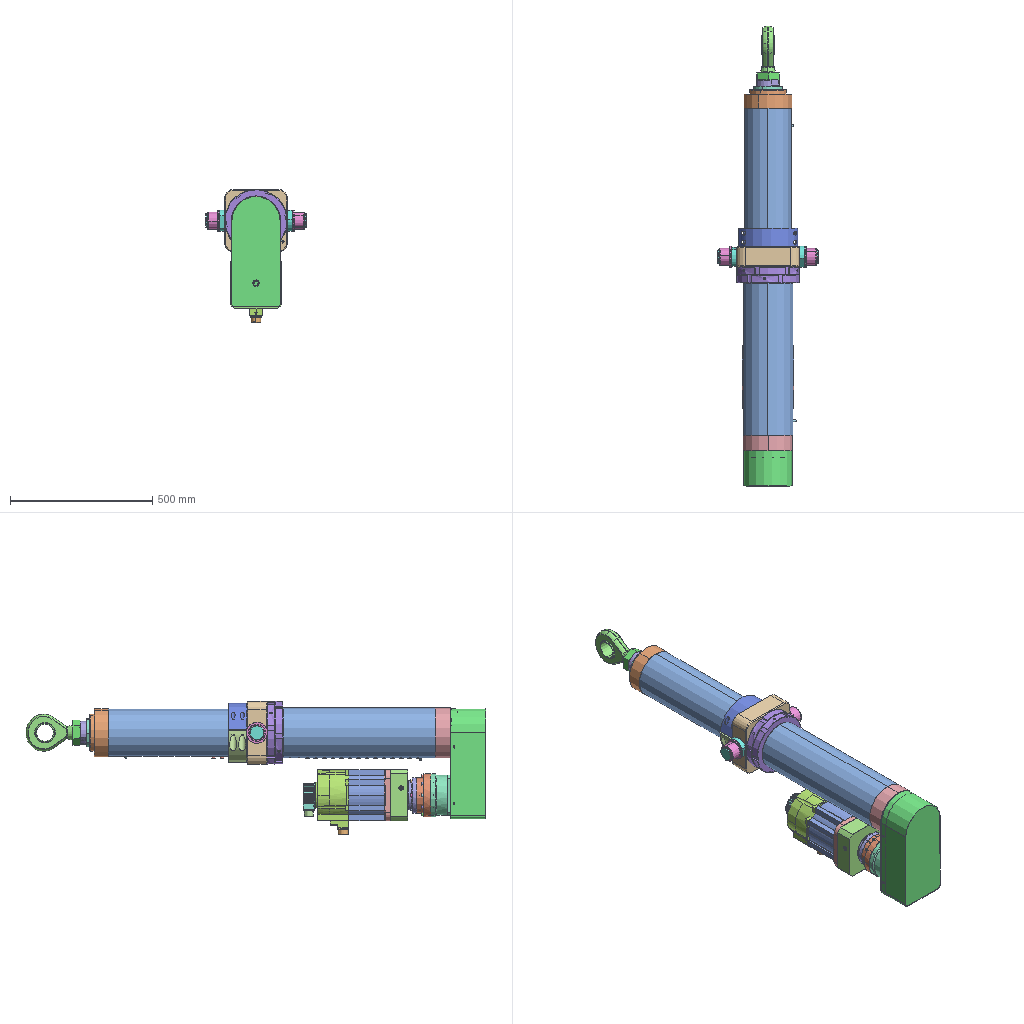Assembly | SolidWorks | 26 different items | 47 placed | box 353 x 1617 x 468 mm
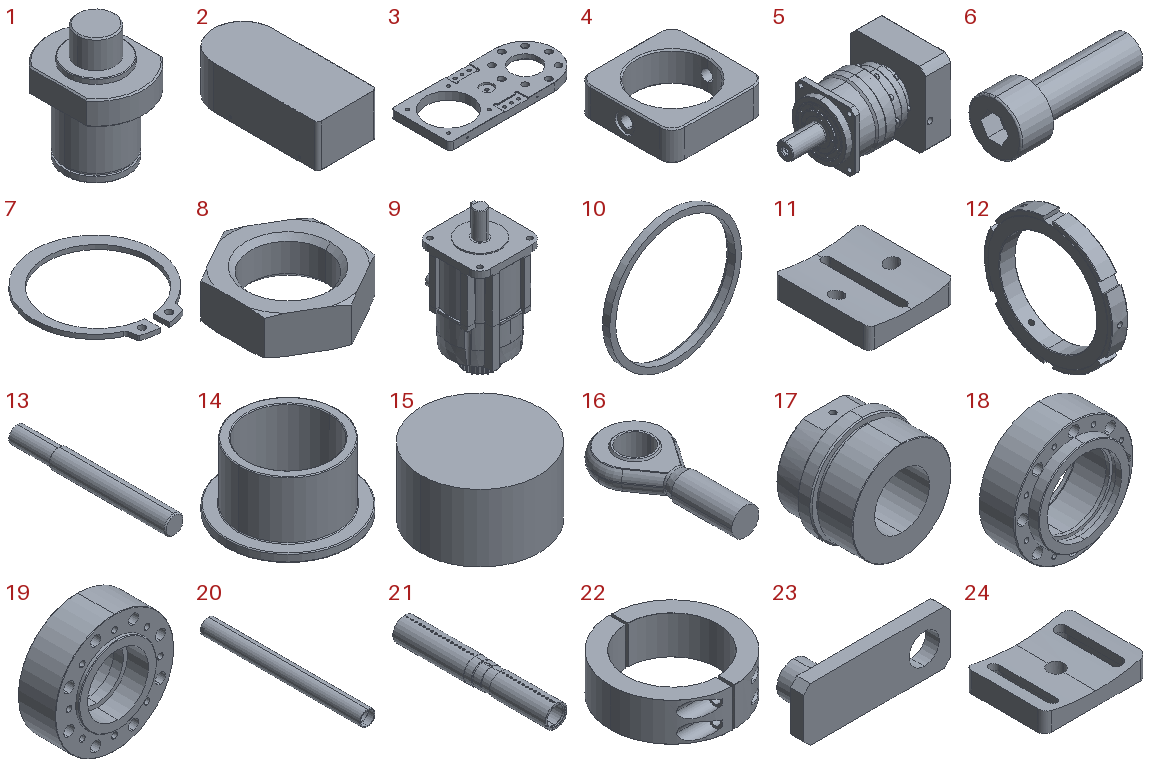Parts list (item | name | quantity | size | volume | features):
1 | - | x2 | 60 x 75 x 92.5 mm | 189510 mm3 | features ICE 7, Chamfer 3, Extrusion 1
2 | - | x1 | 172.4 x 388.4 x 123 mm | 228799 mm3 | features Fillet 2, ICE 2, Extrusion 1
3 | - | x1 | 384.5 x 169 x 23 mm | 899226 mm3 | features HoleWzd 7, ICE 7, MirrorPattern 5, Chamfer 2, CirPattern 1, Extrusion 1, Fillet 1
4 | - | x1 | 220 x 220 x 70 mm | 1778957 mm3 | features ICE 3, Chamfer 1, Extrusion 1, Fillet 1, HoleWzd 1, MirrorPattern 1
5 | - | x1 | 309 x 180 x 180 mm | 4002627 mm3 | features BaseBody 51
6 | - | x16 | 33 x 13 x 13 mm | 2188 mm3 | features BlendCut 1, Cut 1, Fillet 1, LPattern 1, RevCut 1, Revolution 1
7 | - | x1 | 54 x 58.103 x 2 mm | 1377 mm3 | features BaseBody 1
8 | - | x1 | 76.6 x 88.249 x 26 mm | 74263 mm3 | features Cut 2, Chamfer 1, Extrusion 1
9 | - | x1 | 180 x 228 x 387 mm | 7070926 mm3 | features BaseBody 19
10 | - | x1 | 110 x 8 x 110 mm | 11358 mm3 | features Revolution 1
11 | - | x1 | 45 x 50 x 11.442 mm | 18116 mm3 | features ICE 2, Extrusion 1, Fillet 1, HoleWzd 1
12 | - | x2 | 28 x 220 x 219.417 mm | 425123 mm3 | features BaseBody 1
13 | - | x3 | 8 x 66 x 8 mm | 3111 mm3 | features Chamfer 1, Extrusion 1, ICE 1
14 | - | x2 | 75 x 75 x 40 mm | 42442 mm3 | features Fillet 3, Extrusion 1, ICE 1
15 | - | x2 | 8.8 x 8.8 x 5 mm | 304.106 mm3 | features Extrusion 1
16 | - | x1 | 130.224 x 277.5 x 52 mm | 678735 mm3 | features BaseBody 1
17 | - | x1 | 90 x 68 x 90 mm | 254922 mm3 | features ICE 14, Chamfer 4, HoleWzd 2, Extrusion 1
18 | - | x1 | 170 x 78 x 170 mm | 615518 mm3 | features ICE 15, Chamfer 3, CirPattern 3, HoleWzd 3, Extrusion 1
19 | - | x1 | 175 x 73 x 175 mm | 1030889 mm3 | features ICE 6, CirPattern 3, HoleWzd 3, Chamfer 2, Extrusion 1
20 | - | x1 | 100 x 1049 x 100 mm | 2893006 mm3 | features ICE 4, Chamfer 1, Extrusion 1
21 | - | x1 | 175 x 1149 x 175 mm | 10647210 mm3 | features ICE 9, HoleWzd 7, Chamfer 2, CirPattern 2, Extrusion 1, LPattern 1
22 | - | x1 | 210 x 209.94 x 65 mm | 894732 mm3 | features ICE 4, MirrorPattern 3, Chamfer 1, Extrusion 1, HoleWzd 1
23 | - | x1 | 22 x 6 x 8 mm | 394.731 mm3 | features ICE 2, Chamfer 1, Extrusion 1
24 | - | x1 | 45 x 35 x 9.032 mm | 7770 mm3 | features ICE 2, Extrusion 1, Fillet 1, HoleWzd 1
25 | hexagon socket head cap screws gb | x1 | - | - | -
26 | plain parallel keys | x1 | - | - | -
Mates (type | each side: item.copy, entity, surface, feature):
Concentric | assembly face | assembly face | 6 times
Coincident | assembly face | assembly face | 6 times
Coincident | assembly face | 3.1 face plane Boss-Extrude1 | 2 times
DistanceDim | 3.1 face plane Boss-Extrude1 | assembly face
Concentric | 3.1 face cylinder Cut-Extrude1 | assembly face
Coincident | 3.1 face plane Boss-Extrude1 | assembly face
Parallel | 3.1 face plane Boss-Extrude1 | assembly face
Coincident | 3.1 edge | 19.1 face cylinder Cut-Extrude1
Coincident | 3.1 face plane Boss-Extrude1 | 19.1 face plane Boss-Extrude1
Width | 2.1 face plane Boss-Extrude1 | 2.1 face plane Boss-Extrude1 | 3.1 face plane Boss-Extrude1 | 3.1 face plane Boss-Extrude1
Coincident | 3.1 face plane Boss-Extrude1 | 2.1 face plane Boss-Extrude1
Slot | 3.1 face cylinder Mirror1 | 2.1 face cylinder Cut-Extrude1
Concentric | 20.1 face cylinder Cut-Extrude11 | 17.1 face cylinder Boss-Extrude3
Coincident | 20.1 face plane Cut-Extrude8 | 17.1 face plane Cut-Extrude4
Concentric | 17.1 face cylinder M52x5.0 Tapped Hole1 | 16.1 face cylinder Input 1
Concentric | 24.1 face cylinder M8x1.0 Tapped Hole1 | 13.1 face cylinder Boss-Extrude1
Concentric | 3.1 face cylinder Cut-Extrude3 | assembly face
Coincident | assembly face | 23.1 face plane Boss-Extrude1
Concentric | assembly face | 23.1 face cylinder Cut-Extrude1
Parallel | assembly face | 23.1 face plane Boss-Extrude1
Concentric | assembly face | 20.1 face cylinder Cut-Extrude10
Coincident | assembly face | 20.1 face plane Boss-Extrude1
Concentric | 20.1 face cylinder Boss-Extrude1 | 10.1 face cylinder Revolve1
Coincident | 18.1 face plane Boss-Extrude4 | 10.1 face plane Revolve1
Concentric | 9.1 face cylinder Input 1 | assembly face | 2 times
Coincident | 9.1 face plane Input 1 | assembly face
Concentric | 21.1 face cylinder Boss-Extrude1 | 20.1 face cylinder Boss-Extrude1
Coincident | 19.1 face plane Boss-Extrude1 | 21.1 face plane Boss-Extrude1
Concentric | 20.1 face cylinder Boss-Extrude1 | 18.1 face cylinder Boss-Extrude1
Concentric | 21.1 face cylinder CirPattern1 | 18.1 face cylinder CirPattern1
Coincident | 21.1 face plane Boss-Extrude1 | 18.1 face plane Boss-Extrude1
Concentric | 21.1 face cylinder G1/8 Tapped Hole1 | 15.1 face cylinder Boss-Extrude1
Tangent | 21.1 face cylinder Boss-Extrude1 | 15.1 face plane Boss-Extrude1
Coincident | 21.1 face plane Hole size (% based on socket head cap screw type)3 | 6.1 face plane Base-Revolve
Slot | 24.1 face plane Cut-Extrude1 | 21.1 face cylinder M4 Tapped Hole3 | 2 times
Concentric | 21.1 face cylinder Boss-Extrude1 | 24.1 face cylinder Boss-Extrude1
Concentric | 21.1 face cylinder G1/8 Tapped Hole1 | 15.2 face cylinder Boss-Extrude1
Concentric | 21.1 face cylinder Boss-Extrude1 | 11.1 face cylinder Boss-Extrude1
Slot | 11.1 face cylinder M8x1.0 Tapped Hole1 | 21.1 face plane Cut-Extrude13 | 2 times
Concentric | 11.1 edge | 13.2 face cylinder Boss-Extrude1
Concentric | 11.1 face cylinder M8x1.0 Tapped Hole1 | 13.3 face cylinder Boss-Extrude1
Coincident | 13.2 face plane Boss-Extrude2 | 13.3 face plane Boss-Extrude2
DistanceDim | 13.2 face plane Boss-Extrude2 | 11.1 face plane Boss-Extrude1
Concentric | 21.1 face cylinder Hole size (% based on socket head cap screw type)3 | 6.2 face cylinder Base-Revolve
Parallel | 2.1 face plane Boss-Extrude1 | 16.1 face plane Input 1
Concentric | 14.1 face cylinder Boss-Extrude1 | 1.1 face cylinder Boss-Extrude3
Coincident | 14.1 face plane Boss-Extrude2 | 1.1 face plane Boss-Extrude4
Concentric | 21.1 face cylinder Cut-Extrude19 | 4.1 face cylinder Cut-Extrude1
Parallel | 2.1 face plane Boss-Extrude1 | 4.1 face plane Boss-Extrude1
Concentric | 1.1 face cylinder Boss-Extrude1 | 4.1 face cylinder Mirror1
Coincident | 1.1 face plane Cut-Extrude2 | 4.1 face plane Boss-Extrude1
Concentric | 14.2 face cylinder Boss-Extrude1 | 1.2 face cylinder Boss-Extrude3
Coincident | 14.2 face plane Boss-Extrude2 | 1.2 face plane Boss-Extrude4
Coincident | 4.1 face plane Boss-Extrude1 | 1.2 face plane Cut-Extrude2
Concentric | 21.1 face cylinder Cut-Extrude20 | 22.1 face cylinder Boss-Extrude1
Coincident | 22.1 face plane Boss-Extrude1 | 4.1 face plane Boss-Extrude1
Concentric | 21.1 face cylinder Boss-Extrude1 | 12.1 face cylinder Input 1
Coincident | 4.1 face plane Boss-Extrude1 | 12.1 face plane Input 1
Concentric | 21.1 face cylinder Boss-Extrude1 | 12.2 face cylinder Input 1
Coincident | 12.1 face plane Input 1 | 12.2 face plane Input 1
Concentric | 16.1 face cylinder Input 1 | 8.1 face cylinder Base-Extrude
Coincident | 17.1 face plane Boss-Extrude1 | 8.1 face plane Base-Extrude
Parallel | 4.1 face plane Boss-Extrude1 | assembly plane | 2 times
Coincident | 21.1 face plane Cut-Extrude28 | 22.1 face plane Boss-Extrude1
Concentric | assembly face | assembly edge
Concentric | 3.1 face cylinder Hole size (% based on socket head cap screw type)3 | 19.1 face cylinder CirPattern2
Concentric | 3.1 face cylinder Cut-Extrude1 | 5.1 face cylinder Stage 1 ring gear with output shaft KS142 outline-1-solid1
Parallel | 2.1 face plane Boss-Extrude1 | 5.1 face plane Motor flange AKB115 D114.3-M12-200F180H61-1-solid1
Coincident | 3.1 face plane Boss-Extrude1 | 5.1 face plane Stage 1 ring gear with output shaft KS142 outline-1-solid1
Concentric | 9.1 face cylinder Input 18 | 5.1 face cylinder Motor flange AKB115 D114.3-M12-200F180H61-1-solid1
Coincident | 9.1 face plane Input 1 | 5.1 face plane Motor flange AKB115 D114.3-M12-200F180H61-1-solid1
Parallel | 9.1 face plane Input 1 | 5.1 face plane Motor flange AKB115 D114.3-M12-200F180H61-1-solid1
Concentric | 19.1 face cylinder CirPattern1 | 21.1 face cylinder M8 Tapped Hole1
Tangent | 21.1 face cylinder Cut-Extrude26 | 15.2 face plane Boss-Extrude1
Concentric | 1.1 face cylinder Cut-Extrude3 | 7.1 face cylinder Input 1
Coincident | 14.1 face plane Boss-Extrude1 | 7.1 face plane Input 1
DistanceDim | 16.1 face plane Input 1 | 8.1 face plane Base-Extrude
Concentric | 4.1 edge | 1.2 face cylinder Boss-Extrude1